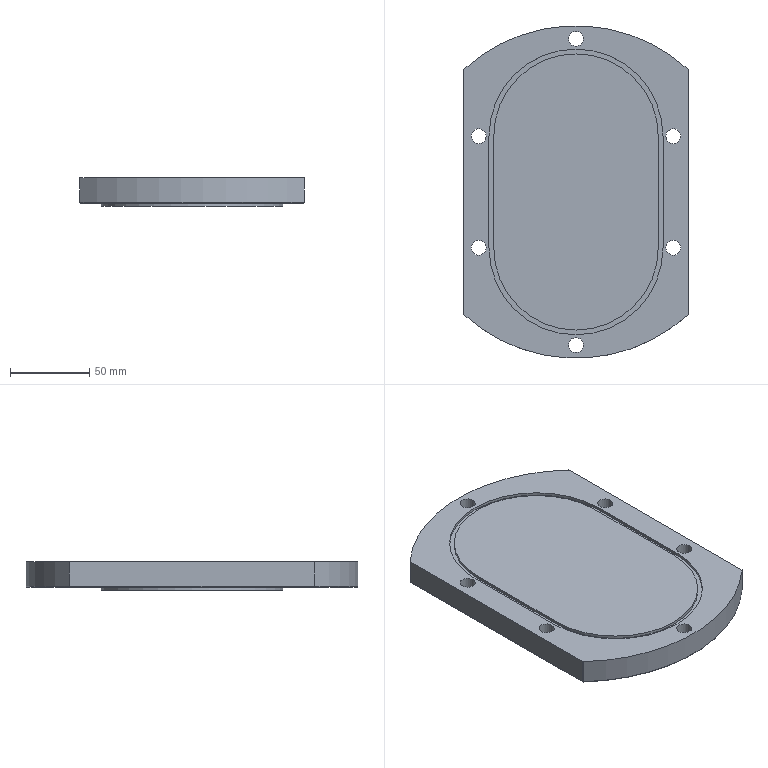Part | 1 solid | 52 faces | box 142 x 210 x 18 mm | volume 444849 mm3 | cylinder 24 | plane 17 | cone 6 | sphere 3 | torus 2 | commonest cylinder face diameters 9.5 x6 14 x6 1 x5 104 x2 110 x2 210 x2
STEP:
#1=CARTESIAN_POINT('',(71.,-77.356,0.));
#2=VERTEX_POINT('',#1);
#3=CARTESIAN_POINT('',(-70.837,-77.505,0.));
#4=VERTEX_POINT('',#3);
#5=CARTESIAN_POINT('',(0.,0.,0.));
#6=DIRECTION('',(0.,0.,-1.));
#7=DIRECTION('',(-1.,0.,0.));
#8=AXIS2_PLACEMENT_3D('',#5,#6,#7);
#9=CIRCLE('',#8,105.);
#10=EDGE_CURVE('',#2,#4,#9,.T.);
#11=ORIENTED_EDGE('',*,*,#10,.T.);
#12=CARTESIAN_POINT('',(-70.837,-77.505,-15.5));
#13=VERTEX_POINT('',#12);
#14=CARTESIAN_POINT('',(-70.837,-77.505,-16.));
#15=DIRECTION('',(0.,0.,1.));
#16=VECTOR('',#15,1000.);
#17=LINE('',#14,#16);
#18=EDGE_CURVE('',#4,#13,#17,.F.);
#19=ORIENTED_EDGE('',*,*,#18,.T.);
#20=CARTESIAN_POINT('',(71.,-77.356,-15.5));
#21=VERTEX_POINT('',#20);
#22=CARTESIAN_POINT('',(0.,0.,-15.5));
#23=DIRECTION('',(0.,0.,-1.));
#24=DIRECTION('',(-1.,0.,0.));
#25=AXIS2_PLACEMENT_3D('',#22,#23,#24);
#26=CIRCLE('',#25,105.);
#27=EDGE_CURVE('',#13,#21,#26,.F.);
#28=ORIENTED_EDGE('',*,*,#27,.T.);
#29=CARTESIAN_POINT('',(71.,-77.356,-16.));
#30=DIRECTION('',(0.,0.,1.));
#31=VECTOR('',#30,1000.);
#32=LINE('',#29,#31);
#33=EDGE_CURVE('',#21,#2,#32,.T.);
#34=ORIENTED_EDGE('',*,*,#33,.T.);
#35=EDGE_LOOP('',(#11,#19,#28,#34));
#36=FACE_BOUND('',#35,.T.);
#37=CARTESIAN_POINT('',(0.,0.,-16.));
#38=DIRECTION('',(0.,0.,1.));
#39=DIRECTION('',(1.,0.,0.));
#40=AXIS2_PLACEMENT_3D('',#37,#38,#39);
#41=CYLINDRICAL_SURFACE('',#40,105.);
#42=ADVANCED_FACE('',(#36),#41,.T.);
#43=CARTESIAN_POINT('',(-71.,-77.136,0.));
#44=VERTEX_POINT('',#43);
#45=CARTESIAN_POINT('',(-71.,77.136,0.));
#46=VERTEX_POINT('',#45);
#47=CARTESIAN_POINT('',(-71.,-77.356,0.));
#48=DIRECTION('',(0.,1.,0.));
#49=VECTOR('',#48,1000.);
#50=LINE('',#47,#49);
#51=EDGE_CURVE('',#44,#46,#50,.T.);
#52=ORIENTED_EDGE('',*,*,#51,.T.);
#53=CARTESIAN_POINT('',(-71.,77.136,-15.5));
#54=VERTEX_POINT('',#53);
#55=CARTESIAN_POINT('',(-71.,77.136,-16.));
#56=DIRECTION('',(0.,0.,1.));
#57=VECTOR('',#56,1000.);
#58=LINE('',#55,#57);
#59=EDGE_CURVE('',#46,#54,#58,.F.);
#60=ORIENTED_EDGE('',*,*,#59,.T.);
#61=CARTESIAN_POINT('',(-71.,-77.136,-15.5));
#62=VERTEX_POINT('',#61);
#63=CARTESIAN_POINT('',(-71.,-77.356,-15.5));
#64=DIRECTION('',(0.,1.,0.));
#65=VECTOR('',#64,1000.);
#66=LINE('',#63,#65);
#67=EDGE_CURVE('',#54,#62,#66,.F.);
#68=ORIENTED_EDGE('',*,*,#67,.T.);
#69=CARTESIAN_POINT('',(-71.,-77.136,-16.));
#70=DIRECTION('',(0.,0.,1.));
#71=VECTOR('',#70,1000.);
#72=LINE('',#69,#71);
#73=EDGE_CURVE('',#62,#44,#72,.T.);
#74=ORIENTED_EDGE('',*,*,#73,.T.);
#75=EDGE_LOOP('',(#52,#60,#68,#74));
#76=FACE_BOUND('',#75,.T.);
#77=CARTESIAN_POINT('',(-71.,-77.356,-16.));
#78=DIRECTION('',(1.,0.,0.));
#79=DIRECTION('',(0.,0.,-1.));
#80=AXIS2_PLACEMENT_3D('',#77,#78,#79);
#81=PLANE('',#80);
#82=ADVANCED_FACE('',(#76),#81,.F.);
#83=CARTESIAN_POINT('',(-70.837,77.505,0.));
#84=VERTEX_POINT('',#83);
#85=CARTESIAN_POINT('',(70.837,77.505,0.));
#86=VERTEX_POINT('',#85);
#87=CARTESIAN_POINT('',(0.,0.,0.));
#88=DIRECTION('',(0.,0.,-1.));
#89=DIRECTION('',(-1.,0.,0.));
#90=AXIS2_PLACEMENT_3D('',#87,#88,#89);
#91=CIRCLE('',#90,105.);
#92=EDGE_CURVE('',#84,#86,#91,.T.);
#93=ORIENTED_EDGE('',*,*,#92,.T.);
#94=CARTESIAN_POINT('',(70.837,77.505,-15.5));
#95=VERTEX_POINT('',#94);
#96=CARTESIAN_POINT('',(70.837,77.505,-16.));
#97=DIRECTION('',(0.,0.,1.));
#98=VECTOR('',#97,1000.);
#99=LINE('',#96,#98);
#100=EDGE_CURVE('',#86,#95,#99,.F.);
#101=ORIENTED_EDGE('',*,*,#100,.T.);
#102=CARTESIAN_POINT('',(-70.837,77.505,-15.5));
#103=VERTEX_POINT('',#102);
#104=CARTESIAN_POINT('',(0.,0.,-15.5));
#105=DIRECTION('',(0.,0.,-1.));
#106=DIRECTION('',(-1.,0.,0.));
#107=AXIS2_PLACEMENT_3D('',#104,#105,#106);
#108=CIRCLE('',#107,105.);
#109=EDGE_CURVE('',#95,#103,#108,.F.);
#110=ORIENTED_EDGE('',*,*,#109,.T.);
#111=CARTESIAN_POINT('',(-70.837,77.505,-16.));
#112=DIRECTION('',(0.,0.,1.));
#113=VECTOR('',#112,1000.);
#114=LINE('',#111,#113);
#115=EDGE_CURVE('',#103,#84,#114,.T.);
#116=ORIENTED_EDGE('',*,*,#115,.T.);
#117=EDGE_LOOP('',(#93,#101,#110,#116));
#118=FACE_BOUND('',#117,.T.);
#119=CARTESIAN_POINT('',(0.,0.,-16.));
#120=DIRECTION('',(0.,0.,1.));
#121=DIRECTION('',(1.,0.,0.));
#122=AXIS2_PLACEMENT_3D('',#119,#120,#121);
#123=CYLINDRICAL_SURFACE('',#122,105.);
#124=ADVANCED_FACE('',(#118),#123,.T.);
#125=CARTESIAN_POINT('',(71.,77.136,-15.5));
#126=VERTEX_POINT('',#125);
#127=CARTESIAN_POINT('',(71.,77.356,-15.5));
#128=DIRECTION('',(0.,-1.,0.));
#129=VECTOR('',#128,1000.);
#130=LINE('',#127,#129);
#131=EDGE_CURVE('',#21,#126,#130,.F.);
#132=ORIENTED_EDGE('',*,*,#131,.T.);
#133=CARTESIAN_POINT('',(71.,77.136,0.));
#134=VERTEX_POINT('',#133);
#135=CARTESIAN_POINT('',(71.,77.136,-16.));
#136=DIRECTION('',(0.,0.,1.));
#137=VECTOR('',#136,1000.);
#138=LINE('',#135,#137);
#139=EDGE_CURVE('',#126,#134,#138,.T.);
#140=ORIENTED_EDGE('',*,*,#139,.T.);
#141=CARTESIAN_POINT('',(71.,77.356,0.));
#142=DIRECTION('',(0.,-1.,0.));
#143=VECTOR('',#142,1000.);
#144=LINE('',#141,#143);
#145=EDGE_CURVE('',#134,#2,#144,.T.);
#146=ORIENTED_EDGE('',*,*,#145,.T.);
#147=ORIENTED_EDGE('',*,*,#33,.F.);
#148=EDGE_LOOP('',(#132,#140,#146,#147));
#149=FACE_BOUND('',#148,.T.);
#150=CARTESIAN_POINT('',(71.,77.356,-16.));
#151=DIRECTION('',(-1.,0.,0.));
#152=DIRECTION('',(0.,0.,1.));
#153=AXIS2_PLACEMENT_3D('',#150,#151,#152);
#154=PLANE('',#153);
#155=ADVANCED_FACE('',(#149),#154,.F.);
#156=CARTESIAN_POINT('',(-70.5,-77.136,-16.));
#157=VERTEX_POINT('',#156);
#158=CARTESIAN_POINT('',(-70.5,77.136,-16.));
#159=VERTEX_POINT('',#158);
#160=CARTESIAN_POINT('',(-70.5,77.356,-16.));
#161=DIRECTION('',(0.,1.,0.));
#162=VECTOR('',#161,1000.);
#163=LINE('',#160,#162);
#164=EDGE_CURVE('',#157,#159,#163,.T.);
#165=ORIENTED_EDGE('',*,*,#164,.T.);
#166=CARTESIAN_POINT('',(70.5,77.136,-16.));
#167=VERTEX_POINT('',#166);
#168=CARTESIAN_POINT('',(0.,0.,-16.));
#169=DIRECTION('',(0.,0.,-1.));
#170=DIRECTION('',(-1.,0.,0.));
#171=AXIS2_PLACEMENT_3D('',#168,#169,#170);
#172=CIRCLE('',#171,104.5);
#173=EDGE_CURVE('',#159,#167,#172,.T.);
#174=ORIENTED_EDGE('',*,*,#173,.T.);
#175=CARTESIAN_POINT('',(70.5,-77.136,-16.));
#176=VERTEX_POINT('',#175);
#177=CARTESIAN_POINT('',(70.5,-77.356,-16.));
#178=DIRECTION('',(0.,-1.,0.));
#179=VECTOR('',#178,1000.);
#180=LINE('',#177,#179);
#181=EDGE_CURVE('',#167,#176,#180,.T.);
#182=ORIENTED_EDGE('',*,*,#181,.T.);
#183=CARTESIAN_POINT('',(0.,0.,-16.));
#184=DIRECTION('',(0.,0.,-1.));
#185=DIRECTION('',(-1.,0.,0.));
#186=AXIS2_PLACEMENT_3D('',#183,#184,#185);
#187=CIRCLE('',#186,104.5);
#188=EDGE_CURVE('',#176,#157,#187,.T.);
#189=ORIENTED_EDGE('',*,*,#188,.T.);
#190=EDGE_LOOP('',(#165,#174,#182,#189));
#191=FACE_BOUND('',#190,.T.);
#192=CARTESIAN_POINT('',(-7.25,96.75,-16.));
#193=VERTEX_POINT('',#192);
#194=CARTESIAN_POINT('',(0.,96.75,-16.));
#195=DIRECTION('',(0.,0.,-1.));
#196=DIRECTION('',(-1.,0.,0.));
#197=AXIS2_PLACEMENT_3D('',#194,#195,#196);
#198=CIRCLE('',#197,7.25);
#199=EDGE_CURVE('',#193,#193,#198,.T.);
#200=ORIENTED_EDGE('',*,*,#199,.F.);
#201=EDGE_LOOP('',(#200));
#202=FACE_BOUND('',#201,.T.);
#203=CARTESIAN_POINT('',(54.25,35.25,-16.));
#204=VERTEX_POINT('',#203);
#205=CARTESIAN_POINT('',(61.5,35.25,-16.));
#206=DIRECTION('',(0.,0.,-1.));
#207=DIRECTION('',(-1.,0.,0.));
#208=AXIS2_PLACEMENT_3D('',#205,#206,#207);
#209=CIRCLE('',#208,7.25);
#210=EDGE_CURVE('',#204,#204,#209,.T.);
#211=ORIENTED_EDGE('',*,*,#210,.F.);
#212=EDGE_LOOP('',(#211));
#213=FACE_BOUND('',#212,.T.);
#214=CARTESIAN_POINT('',(-68.75,35.25,-16.));
#215=VERTEX_POINT('',#214);
#216=CARTESIAN_POINT('',(-61.5,35.25,-16.));
#217=DIRECTION('',(0.,0.,-1.));
#218=DIRECTION('',(-1.,0.,0.));
#219=AXIS2_PLACEMENT_3D('',#216,#217,#218);
#220=CIRCLE('',#219,7.25);
#221=EDGE_CURVE('',#215,#215,#220,.T.);
#222=ORIENTED_EDGE('',*,*,#221,.F.);
#223=EDGE_LOOP('',(#222));
#224=FACE_BOUND('',#223,.T.);
#225=CARTESIAN_POINT('',(-68.75,-35.25,-16.));
#226=VERTEX_POINT('',#225);
#227=CARTESIAN_POINT('',(-61.5,-35.25,-16.));
#228=DIRECTION('',(0.,0.,-1.));
#229=DIRECTION('',(-1.,0.,0.));
#230=AXIS2_PLACEMENT_3D('',#227,#228,#229);
#231=CIRCLE('',#230,7.25);
#232=EDGE_CURVE('',#226,#226,#231,.T.);
#233=ORIENTED_EDGE('',*,*,#232,.F.);
#234=EDGE_LOOP('',(#233));
#235=FACE_BOUND('',#234,.T.);
#236=CARTESIAN_POINT('',(54.25,-35.25,-16.));
#237=VERTEX_POINT('',#236);
#238=CARTESIAN_POINT('',(61.5,-35.25,-16.));
#239=DIRECTION('',(0.,0.,-1.));
#240=DIRECTION('',(-1.,0.,0.));
#241=AXIS2_PLACEMENT_3D('',#238,#239,#240);
#242=CIRCLE('',#241,7.25);
#243=EDGE_CURVE('',#237,#237,#242,.T.);
#244=ORIENTED_EDGE('',*,*,#243,.F.);
#245=EDGE_LOOP('',(#244));
#246=FACE_BOUND('',#245,.T.);
#247=CARTESIAN_POINT('',(-7.25,-96.75,-16.));
#248=VERTEX_POINT('',#247);
#249=CARTESIAN_POINT('',(0.,-96.75,-16.));
#250=DIRECTION('',(0.,0.,-1.));
#251=DIRECTION('',(-1.,0.,0.));
#252=AXIS2_PLACEMENT_3D('',#249,#250,#251);
#253=CIRCLE('',#252,7.25);
#254=EDGE_CURVE('',#248,#248,#253,.T.);
#255=ORIENTED_EDGE('',*,*,#254,.F.);
#256=EDGE_LOOP('',(#255));
#257=FACE_BOUND('',#256,.T.);
#258=CARTESIAN_POINT('',(-57.5,0.,-16.));
#259=VERTEX_POINT('',#258);
#260=CARTESIAN_POINT('',(0.,0.,-16.));
#261=DIRECTION('',(0.,0.,-1.));
#262=DIRECTION('',(-1.,0.,0.));
#263=AXIS2_PLACEMENT_3D('',#260,#261,#262);
#264=CIRCLE('',#263,57.5);
#265=EDGE_CURVE('',#259,#259,#264,.T.);
#266=ORIENTED_EDGE('',*,*,#265,.F.);
#267=EDGE_LOOP('',(#266));
#268=FACE_BOUND('',#267,.T.);
#269=CARTESIAN_POINT('',(0.,0.,-16.));
#270=DIRECTION('',(0.,0.,-1.));
#271=DIRECTION('',(-1.,0.,0.));
#272=AXIS2_PLACEMENT_3D('',#269,#270,#271);
#273=PLANE('',#272);
#274=ADVANCED_FACE('',(#191,#202,#213,#224,#235,#246,#257,#268),#273,.T.);
#275=CARTESIAN_POINT('',(-55.,35.25,0.));
#276=VERTEX_POINT('',#275);
#277=CARTESIAN_POINT('',(-55.,-35.25,0.));
#278=VERTEX_POINT('',#277);
#279=CARTESIAN_POINT('',(-55.,35.25,0.));
#280=DIRECTION('',(0.,-1.,0.));
#281=VECTOR('',#280,1000.);
#282=LINE('',#279,#281);
#283=EDGE_CURVE('',#276,#278,#282,.T.);
#284=ORIENTED_EDGE('',*,*,#283,.F.);
#285=CARTESIAN_POINT('',(55.,35.25,0.));
#286=VERTEX_POINT('',#285);
#287=CARTESIAN_POINT('',(0.,35.25,0.));
#288=DIRECTION('',(0.,0.,1.));
#289=DIRECTION('',(1.,0.,0.));
#290=AXIS2_PLACEMENT_3D('',#287,#288,#289);
#291=CIRCLE('',#290,55.);
#292=EDGE_CURVE('',#286,#276,#291,.T.);
#293=ORIENTED_EDGE('',*,*,#292,.F.);
#294=CARTESIAN_POINT('',(55.,-35.25,0.));
#295=VERTEX_POINT('',#294);
#296=CARTESIAN_POINT('',(55.,35.25,0.));
#297=DIRECTION('',(0.,1.,0.));
#298=VECTOR('',#297,1000.);
#299=LINE('',#296,#298);
#300=EDGE_CURVE('',#295,#286,#299,.T.);
#301=ORIENTED_EDGE('',*,*,#300,.F.);
#302=CARTESIAN_POINT('',(0.,-35.25,0.));
#303=DIRECTION('',(0.,0.,1.));
#304=DIRECTION('',(1.,0.,0.));
#305=AXIS2_PLACEMENT_3D('',#302,#303,#304);
#306=CIRCLE('',#305,55.);
#307=EDGE_CURVE('',#278,#295,#306,.T.);
#308=ORIENTED_EDGE('',*,*,#307,.F.);
#309=EDGE_LOOP('',(#284,#293,#301,#308));
#310=FACE_BOUND('',#309,.T.);
#311=CARTESIAN_POINT('',(-4.75,96.75,0.));
#312=VERTEX_POINT('',#311);
#313=CARTESIAN_POINT('',(0.,96.75,0.));
#314=DIRECTION('',(0.,0.,-1.));
#315=DIRECTION('',(-1.,0.,0.));
#316=AXIS2_PLACEMENT_3D('',#313,#314,#315);
#317=CIRCLE('',#316,4.75);
#318=EDGE_CURVE('',#312,#312,#317,.T.);
#319=ORIENTED_EDGE('',*,*,#318,.T.);
#320=EDGE_LOOP('',(#319));
#321=FACE_BOUND('',#320,.T.);
#322=CARTESIAN_POINT('',(56.75,35.25,0.));
#323=VERTEX_POINT('',#322);
#324=CARTESIAN_POINT('',(61.5,35.25,0.));
#325=DIRECTION('',(0.,0.,-1.));
#326=DIRECTION('',(-1.,0.,0.));
#327=AXIS2_PLACEMENT_3D('',#324,#325,#326);
#328=CIRCLE('',#327,4.75);
#329=EDGE_CURVE('',#323,#323,#328,.T.);
#330=ORIENTED_EDGE('',*,*,#329,.T.);
#331=EDGE_LOOP('',(#330));
#332=FACE_BOUND('',#331,.T.);
#333=CARTESIAN_POINT('',(-66.25,35.25,0.));
#334=VERTEX_POINT('',#333);
#335=CARTESIAN_POINT('',(-61.5,35.25,0.));
#336=DIRECTION('',(0.,0.,-1.));
#337=DIRECTION('',(-1.,0.,0.));
#338=AXIS2_PLACEMENT_3D('',#335,#336,#337);
#339=CIRCLE('',#338,4.75);
#340=EDGE_CURVE('',#334,#334,#339,.T.);
#341=ORIENTED_EDGE('',*,*,#340,.T.);
#342=EDGE_LOOP('',(#341));
#343=FACE_BOUND('',#342,.T.);
#344=CARTESIAN_POINT('',(-66.25,-35.25,0.));
#345=VERTEX_POINT('',#344);
#346=CARTESIAN_POINT('',(-61.5,-35.25,0.));
#347=DIRECTION('',(0.,0.,-1.));
#348=DIRECTION('',(-1.,0.,0.));
#349=AXIS2_PLACEMENT_3D('',#346,#347,#348);
#350=CIRCLE('',#349,4.75);
#351=EDGE_CURVE('',#345,#345,#350,.T.);
#352=ORIENTED_EDGE('',*,*,#351,.T.);
#353=EDGE_LOOP('',(#352));
#354=FACE_BOUND('',#353,.T.);
#355=CARTESIAN_POINT('',(56.75,-35.25,0.));
#356=VERTEX_POINT('',#355);
#357=CARTESIAN_POINT('',(61.5,-35.25,0.));
#358=DIRECTION('',(0.,0.,-1.));
#359=DIRECTION('',(-1.,0.,0.));
#360=AXIS2_PLACEMENT_3D('',#357,#358,#359);
#361=CIRCLE('',#360,4.75);
#362=EDGE_CURVE('',#356,#356,#361,.T.);
#363=ORIENTED_EDGE('',*,*,#362,.T.);
#364=EDGE_LOOP('',(#363));
#365=FACE_BOUND('',#364,.T.);
#366=CARTESIAN_POINT('',(-4.75,-96.75,0.));
#367=VERTEX_POINT('',#366);
#368=CARTESIAN_POINT('',(0.,-96.75,0.));
#369=DIRECTION('',(0.,0.,-1.));
#370=DIRECTION('',(-1.,0.,0.));
#371=AXIS2_PLACEMENT_3D('',#368,#369,#370);
#372=CIRCLE('',#371,4.75);
#373=EDGE_CURVE('',#367,#367,#372,.T.);
#374=ORIENTED_EDGE('',*,*,#373,.T.);
#375=EDGE_LOOP('',(#374));
#376=FACE_BOUND('',#375,.T.);
#377=ORIENTED_EDGE('',*,*,#145,.F.);
#378=CARTESIAN_POINT('',(70.5,77.136,0.));
#379=DIRECTION('',(0.,0.,-1.));
#380=DIRECTION('',(-1.,0.,0.));
#381=AXIS2_PLACEMENT_3D('',#378,#379,#380);
#382=CIRCLE('',#381,0.5);
#383=EDGE_CURVE('',#134,#86,#382,.F.);
#384=ORIENTED_EDGE('',*,*,#383,.T.);
#385=ORIENTED_EDGE('',*,*,#92,.F.);
#386=CARTESIAN_POINT('',(-70.5,77.136,0.));
#387=DIRECTION('',(0.,0.,-1.));
#388=DIRECTION('',(-1.,0.,0.));
#389=AXIS2_PLACEMENT_3D('',#386,#387,#388);
#390=CIRCLE('',#389,0.5);
#391=EDGE_CURVE('',#84,#46,#390,.F.);
#392=ORIENTED_EDGE('',*,*,#391,.T.);
#393=ORIENTED_EDGE('',*,*,#51,.F.);
#394=CARTESIAN_POINT('',(-70.5,-77.136,0.));
#395=DIRECTION('',(0.,0.,-1.));
#396=DIRECTION('',(-1.,0.,0.));
#397=AXIS2_PLACEMENT_3D('',#394,#395,#396);
#398=CIRCLE('',#397,0.5);
#399=EDGE_CURVE('',#44,#4,#398,.F.);
#400=ORIENTED_EDGE('',*,*,#399,.T.);
#401=ORIENTED_EDGE('',*,*,#10,.F.);
#402=EDGE_LOOP('',(#377,#384,#385,#392,#393,#400,#401));
#403=FACE_BOUND('',#402,.T.);
#404=CARTESIAN_POINT('',(0.,0.,0.));
#405=DIRECTION('',(0.,0.,-1.));
#406=DIRECTION('',(-1.,0.,0.));
#407=AXIS2_PLACEMENT_3D('',#404,#405,#406);
#408=PLANE('',#407);
#409=ADVANCED_FACE('',(#310,#321,#332,#343,#354,#365,#376,#403),#408,.F.);
#410=CARTESIAN_POINT('',(-57.5,0.,-18.));
#411=VERTEX_POINT('',#410);
#412=CARTESIAN_POINT('',(0.,0.,-18.));
#413=DIRECTION('',(0.,0.,-1.));
#414=DIRECTION('',(-1.,0.,0.));
#415=AXIS2_PLACEMENT_3D('',#412,#413,#414);
#416=CIRCLE('',#415,57.5);
#417=EDGE_CURVE('',#411,#411,#416,.T.);
#418=ORIENTED_EDGE('',*,*,#417,.F.);
#419=EDGE_LOOP('',(#418));
#420=FACE_BOUND('',#419,.T.);
#421=ORIENTED_EDGE('',*,*,#265,.T.);
#422=EDGE_LOOP('',(#421));
#423=FACE_BOUND('',#422,.T.);
#424=CARTESIAN_POINT('',(0.,0.,-18.));
#425=DIRECTION('',(0.,0.,1.));
#426=DIRECTION('',(1.,0.,0.));
#427=AXIS2_PLACEMENT_3D('',#424,#425,#426);
#428=CYLINDRICAL_SURFACE('',#427,57.5);
#429=ADVANCED_FACE('',(#420,#423),#428,.T.);
#430=ORIENTED_EDGE('',*,*,#417,.T.);
#431=EDGE_LOOP('',(#430));
#432=FACE_BOUND('',#431,.T.);
#433=CARTESIAN_POINT('',(0.,0.,-18.));
#434=DIRECTION('',(0.,0.,-1.));
#435=DIRECTION('',(-1.,0.,0.));
#436=AXIS2_PLACEMENT_3D('',#433,#434,#435);
#437=PLANE('',#436);
#438=ADVANCED_FACE('',(#432),#437,.T.);
#439=CARTESIAN_POINT('',(-4.75,-96.75,-7.5));
#440=VERTEX_POINT('',#439);
#441=CARTESIAN_POINT('',(0.,-96.75,-7.5));
#442=DIRECTION('',(0.,0.,-1.));
#443=DIRECTION('',(-1.,0.,0.));
#444=AXIS2_PLACEMENT_3D('',#441,#442,#443);
#445=CIRCLE('',#444,4.75);
#446=EDGE_CURVE('',#440,#440,#445,.T.);
#447=ORIENTED_EDGE('',*,*,#446,.T.);
#448=EDGE_LOOP('',(#447));
#449=FACE_BOUND('',#448,.T.);
#450=ORIENTED_EDGE('',*,*,#373,.F.);
#451=EDGE_LOOP('',(#450));
#452=FACE_BOUND('',#451,.T.);
#453=CARTESIAN_POINT('',(0.,-96.75,-16.));
#454=DIRECTION('',(0.,0.,-1.));
#455=DIRECTION('',(-1.,0.,0.));
#456=AXIS2_PLACEMENT_3D('',#453,#454,#455);
#457=CYLINDRICAL_SURFACE('',#456,4.75);
#458=ADVANCED_FACE('',(#449,#452),#457,.F.);
#459=ORIENTED_EDGE('',*,*,#446,.F.);
#460=EDGE_LOOP('',(#459));
#461=FACE_BOUND('',#460,.T.);
#462=CARTESIAN_POINT('',(-7.,-96.75,-7.5));
#463=VERTEX_POINT('',#462);
#464=CARTESIAN_POINT('',(0.,-96.75,-7.5));
#465=DIRECTION('',(0.,0.,-1.));
#466=DIRECTION('',(-1.,0.,0.));
#467=AXIS2_PLACEMENT_3D('',#464,#465,#466);
#468=CIRCLE('',#467,7.);
#469=EDGE_CURVE('',#463,#463,#468,.T.);
#470=ORIENTED_EDGE('',*,*,#469,.T.);
#471=EDGE_LOOP('',(#470));
#472=FACE_BOUND('',#471,.T.);
#473=CARTESIAN_POINT('',(-4.75,-96.75,-7.5));
#474=DIRECTION('',(0.,0.,1.));
#475=DIRECTION('',(1.,0.,0.));
#476=AXIS2_PLACEMENT_3D('',#473,#474,#475);
#477=PLANE('',#476);
#478=ADVANCED_FACE('',(#461,#472),#477,.F.);
#479=ORIENTED_EDGE('',*,*,#469,.F.);
#480=EDGE_LOOP('',(#479));
#481=FACE_BOUND('',#480,.T.);
#482=CARTESIAN_POINT('',(-7.,-96.75,-15.75));
#483=VERTEX_POINT('',#482);
#484=CARTESIAN_POINT('',(0.,-96.75,-15.75));
#485=DIRECTION('',(0.,0.,-1.));
#486=DIRECTION('',(-1.,0.,0.));
#487=AXIS2_PLACEMENT_3D('',#484,#485,#486);
#488=CIRCLE('',#487,7.);
#489=EDGE_CURVE('',#483,#483,#488,.T.);
#490=ORIENTED_EDGE('',*,*,#489,.T.);
#491=EDGE_LOOP('',(#490));
#492=FACE_BOUND('',#491,.T.);
#493=CARTESIAN_POINT('',(0.,-96.75,-16.));
#494=DIRECTION('',(0.,0.,-1.));
#495=DIRECTION('',(-1.,0.,0.));
#496=AXIS2_PLACEMENT_3D('',#493,#494,#495);
#497=CYLINDRICAL_SURFACE('',#496,7.);
#498=ADVANCED_FACE('',(#481,#492),#497,.F.);
#499=ORIENTED_EDGE('',*,*,#489,.F.);
#500=EDGE_LOOP('',(#499));
#501=FACE_BOUND('',#500,.T.);
#502=ORIENTED_EDGE('',*,*,#254,.T.);
#503=EDGE_LOOP('',(#502));
#504=FACE_BOUND('',#503,.T.);
#505=CARTESIAN_POINT('',(0.,-96.75,-16.));
#506=DIRECTION('',(0.,0.,-1.));
#507=DIRECTION('',(-1.,0.,0.));
#508=AXIS2_PLACEMENT_3D('',#505,#506,#507);
#509=CONICAL_SURFACE('',#508,7.25,0.7854);
#510=ADVANCED_FACE('',(#501,#504),#509,.F.);
#511=CARTESIAN_POINT('',(56.75,-35.25,-7.5));
#512=VERTEX_POINT('',#511);
#513=CARTESIAN_POINT('',(61.5,-35.25,-7.5));
#514=DIRECTION('',(0.,0.,-1.));
#515=DIRECTION('',(-1.,0.,0.));
#516=AXIS2_PLACEMENT_3D('',#513,#514,#515);
#517=CIRCLE('',#516,4.75);
#518=EDGE_CURVE('',#512,#512,#517,.T.);
#519=ORIENTED_EDGE('',*,*,#518,.T.);
#520=EDGE_LOOP('',(#519));
#521=FACE_BOUND('',#520,.T.);
#522=ORIENTED_EDGE('',*,*,#362,.F.);
#523=EDGE_LOOP('',(#522));
#524=FACE_BOUND('',#523,.T.);
#525=CARTESIAN_POINT('',(61.5,-35.25,-16.));
#526=DIRECTION('',(0.,0.,-1.));
#527=DIRECTION('',(-1.,0.,0.));
#528=AXIS2_PLACEMENT_3D('',#525,#526,#527);
#529=CYLINDRICAL_SURFACE('',#528,4.75);
#530=ADVANCED_FACE('',(#521,#524),#529,.F.);
#531=ORIENTED_EDGE('',*,*,#518,.F.);
#532=EDGE_LOOP('',(#531));
#533=FACE_BOUND('',#532,.T.);
#534=CARTESIAN_POINT('',(54.5,-35.25,-7.5));
#535=VERTEX_POINT('',#534);
#536=CARTESIAN_POINT('',(61.5,-35.25,-7.5));
#537=DIRECTION('',(0.,0.,-1.));
#538=DIRECTION('',(-1.,0.,0.));
#539=AXIS2_PLACEMENT_3D('',#536,#537,#538);
#540=CIRCLE('',#539,7.);
#541=EDGE_CURVE('',#535,#535,#540,.T.);
#542=ORIENTED_EDGE('',*,*,#541,.T.);
#543=EDGE_LOOP('',(#542));
#544=FACE_BOUND('',#543,.T.);
#545=CARTESIAN_POINT('',(56.75,-35.25,-7.5));
#546=DIRECTION('',(0.,0.,1.));
#547=DIRECTION('',(1.,0.,0.));
#548=AXIS2_PLACEMENT_3D('',#545,#546,#547);
#549=PLANE('',#548);
#550=ADVANCED_FACE('',(#533,#544),#549,.F.);
#551=ORIENTED_EDGE('',*,*,#541,.F.);
#552=EDGE_LOOP('',(#551));
#553=FACE_BOUND('',#552,.T.);
#554=CARTESIAN_POINT('',(54.5,-35.25,-15.75));
#555=VERTEX_POINT('',#554);
#556=CARTESIAN_POINT('',(61.5,-35.25,-15.75));
#557=DIRECTION('',(0.,0.,-1.));
#558=DIRECTION('',(-1.,0.,0.));
#559=AXIS2_PLACEMENT_3D('',#556,#557,#558);
#560=CIRCLE('',#559,7.);
#561=EDGE_CURVE('',#555,#555,#560,.T.);
#562=ORIENTED_EDGE('',*,*,#561,.T.);
#563=EDGE_LOOP('',(#562));
#564=FACE_BOUND('',#563,.T.);
#565=CARTESIAN_POINT('',(61.5,-35.25,-16.));
#566=DIRECTION('',(0.,0.,-1.));
#567=DIRECTION('',(-1.,0.,0.));
#568=AXIS2_PLACEMENT_3D('',#565,#566,#567);
#569=CYLINDRICAL_SURFACE('',#568,7.);
#570=ADVANCED_FACE('',(#553,#564),#569,.F.);
#571=ORIENTED_EDGE('',*,*,#561,.F.);
#572=EDGE_LOOP('',(#571));
#573=FACE_BOUND('',#572,.T.);
#574=ORIENTED_EDGE('',*,*,#243,.T.);
#575=EDGE_LOOP('',(#574));
#576=FACE_BOUND('',#575,.T.);
#577=CARTESIAN_POINT('',(61.5,-35.25,-16.));
#578=DIRECTION('',(0.,0.,-1.));
#579=DIRECTION('',(-1.,0.,0.));
#580=AXIS2_PLACEMENT_3D('',#577,#578,#579);
#581=CONICAL_SURFACE('',#580,7.25,0.7854);
#582=ADVANCED_FACE('',(#573,#576),#581,.F.);
#583=CARTESIAN_POINT('',(-66.25,-35.25,-7.5));
#584=VERTEX_POINT('',#583);
#585=CARTESIAN_POINT('',(-61.5,-35.25,-7.5));
#586=DIRECTION('',(0.,0.,-1.));
#587=DIRECTION('',(-1.,0.,0.));
#588=AXIS2_PLACEMENT_3D('',#585,#586,#587);
#589=CIRCLE('',#588,4.75);
#590=EDGE_CURVE('',#584,#584,#589,.T.);
#591=ORIENTED_EDGE('',*,*,#590,.T.);
#592=EDGE_LOOP('',(#591));
#593=FACE_BOUND('',#592,.T.);
#594=ORIENTED_EDGE('',*,*,#351,.F.);
#595=EDGE_LOOP('',(#594));
#596=FACE_BOUND('',#595,.T.);
#597=CARTESIAN_POINT('',(-61.5,-35.25,-16.));
#598=DIRECTION('',(0.,0.,-1.));
#599=DIRECTION('',(-1.,0.,0.));
#600=AXIS2_PLACEMENT_3D('',#597,#598,#599);
#601=CYLINDRICAL_SURFACE('',#600,4.75);
#602=ADVANCED_FACE('',(#593,#596),#601,.F.);
#603=ORIENTED_EDGE('',*,*,#590,.F.);
#604=EDGE_LOOP('',(#603));
#605=FACE_BOUND('',#604,.T.);
#606=CARTESIAN_POINT('',(-68.5,-35.25,-7.5));
#607=VERTEX_POINT('',#606);
#608=CARTESIAN_POINT('',(-61.5,-35.25,-7.5));
#609=DIRECTION('',(0.,0.,-1.));
#610=DIRECTION('',(-1.,0.,0.));
#611=AXIS2_PLACEMENT_3D('',#608,#609,#610);
#612=CIRCLE('',#611,7.);
#613=EDGE_CURVE('',#607,#607,#612,.T.);
#614=ORIENTED_EDGE('',*,*,#613,.T.);
#615=EDGE_LOOP('',(#614));
#616=FACE_BOUND('',#615,.T.);
#617=CARTESIAN_POINT('',(-66.25,-35.25,-7.5));
#618=DIRECTION('',(0.,0.,1.));
#619=DIRECTION('',(1.,0.,0.));
#620=AXIS2_PLACEMENT_3D('',#617,#618,#619);
#621=PLANE('',#620);
#622=ADVANCED_FACE('',(#605,#616),#621,.F.);
#623=ORIENTED_EDGE('',*,*,#613,.F.);
#624=EDGE_LOOP('',(#623));
#625=FACE_BOUND('',#624,.T.);
#626=CARTESIAN_POINT('',(-68.5,-35.25,-15.75));
#627=VERTEX_POINT('',#626);
#628=CARTESIAN_POINT('',(-61.5,-35.25,-15.75));
#629=DIRECTION('',(0.,0.,-1.));
#630=DIRECTION('',(-1.,0.,0.));
#631=AXIS2_PLACEMENT_3D('',#628,#629,#630);
#632=CIRCLE('',#631,7.);
#633=EDGE_CURVE('',#627,#627,#632,.T.);
#634=ORIENTED_EDGE('',*,*,#633,.T.);
#635=EDGE_LOOP('',(#634));
#636=FACE_BOUND('',#635,.T.);
#637=CARTESIAN_POINT('',(-61.5,-35.25,-16.));
#638=DIRECTION('',(0.,0.,-1.));
#639=DIRECTION('',(-1.,0.,0.));
#640=AXIS2_PLACEMENT_3D('',#637,#638,#639);
#641=CYLINDRICAL_SURFACE('',#640,7.);
#642=ADVANCED_FACE('',(#625,#636),#641,.F.);
#643=ORIENTED_EDGE('',*,*,#633,.F.);
#644=EDGE_LOOP('',(#643));
#645=FACE_BOUND('',#644,.T.);
#646=ORIENTED_EDGE('',*,*,#232,.T.);
#647=EDGE_LOOP('',(#646));
#648=FACE_BOUND('',#647,.T.);
#649=CARTESIAN_POINT('',(-61.5,-35.25,-16.));
#650=DIRECTION('',(0.,0.,-1.));
#651=DIRECTION('',(-1.,0.,0.));
#652=AXIS2_PLACEMENT_3D('',#649,#650,#651);
#653=CONICAL_SURFACE('',#652,7.25,0.7854);
#654=ADVANCED_FACE('',(#645,#648),#653,.F.);
#655=CARTESIAN_POINT('',(-66.25,35.25,-7.5));
#656=VERTEX_POINT('',#655);
#657=CARTESIAN_POINT('',(-61.5,35.25,-7.5));
#658=DIRECTION('',(0.,0.,-1.));
#659=DIRECTION('',(-1.,0.,0.));
#660=AXIS2_PLACEMENT_3D('',#657,#658,#659);
#661=CIRCLE('',#660,4.75);
#662=EDGE_CURVE('',#656,#656,#661,.T.);
#663=ORIENTED_EDGE('',*,*,#662,.T.);
#664=EDGE_LOOP('',(#663));
#665=FACE_BOUND('',#664,.T.);
#666=ORIENTED_EDGE('',*,*,#340,.F.);
#667=EDGE_LOOP('',(#666));
#668=FACE_BOUND('',#667,.T.);
#669=CARTESIAN_POINT('',(-61.5,35.25,-16.));
#670=DIRECTION('',(0.,0.,-1.));
#671=DIRECTION('',(-1.,0.,0.));
#672=AXIS2_PLACEMENT_3D('',#669,#670,#671);
#673=CYLINDRICAL_SURFACE('',#672,4.75);
#674=ADVANCED_FACE('',(#665,#668),#673,.F.);
#675=ORIENTED_EDGE('',*,*,#662,.F.);
#676=EDGE_LOOP('',(#675));
#677=FACE_BOUND('',#676,.T.);
#678=CARTESIAN_POINT('',(-68.5,35.25,-7.5));
#679=VERTEX_POINT('',#678);
#680=CARTESIAN_POINT('',(-61.5,35.25,-7.5));
#681=DIRECTION('',(0.,0.,-1.));
#682=DIRECTION('',(-1.,0.,0.));
#683=AXIS2_PLACEMENT_3D('',#680,#681,#682);
#684=CIRCLE('',#683,7.);
#685=EDGE_CURVE('',#679,#679,#684,.T.);
#686=ORIENTED_EDGE('',*,*,#685,.T.);
#687=EDGE_LOOP('',(#686));
#688=FACE_BOUND('',#687,.T.);
#689=CARTESIAN_POINT('',(-66.25,35.25,-7.5));
#690=DIRECTION('',(0.,0.,1.));
#691=DIRECTION('',(1.,0.,0.));
#692=AXIS2_PLACEMENT_3D('',#689,#690,#691);
#693=PLANE('',#692);
#694=ADVANCED_FACE('',(#677,#688),#693,.F.);
#695=ORIENTED_EDGE('',*,*,#685,.F.);
#696=EDGE_LOOP('',(#695));
#697=FACE_BOUND('',#696,.T.);
#698=CARTESIAN_POINT('',(-68.5,35.25,-15.75));
#699=VERTEX_POINT('',#698);
#700=CARTESIAN_POINT('',(-61.5,35.25,-15.75));
#701=DIRECTION('',(0.,0.,-1.));
#702=DIRECTION('',(-1.,0.,0.));
#703=AXIS2_PLACEMENT_3D('',#700,#701,#702);
#704=CIRCLE('',#703,7.);
#705=EDGE_CURVE('',#699,#699,#704,.T.);
#706=ORIENTED_EDGE('',*,*,#705,.T.);
#707=EDGE_LOOP('',(#706));
#708=FACE_BOUND('',#707,.T.);
#709=CARTESIAN_POINT('',(-61.5,35.25,-16.));
#710=DIRECTION('',(0.,0.,-1.));
#711=DIRECTION('',(-1.,0.,0.));
#712=AXIS2_PLACEMENT_3D('',#709,#710,#711);
#713=CYLINDRICAL_SURFACE('',#712,7.);
#714=ADVANCED_FACE('',(#697,#708),#713,.F.);
#715=ORIENTED_EDGE('',*,*,#705,.F.);
#716=EDGE_LOOP('',(#715));
#717=FACE_BOUND('',#716,.T.);
#718=ORIENTED_EDGE('',*,*,#221,.T.);
#719=EDGE_LOOP('',(#718));
#720=FACE_BOUND('',#719,.T.);
#721=CARTESIAN_POINT('',(-61.5,35.25,-16.));
#722=DIRECTION('',(0.,0.,-1.));
#723=DIRECTION('',(-1.,0.,0.));
#724=AXIS2_PLACEMENT_3D('',#721,#722,#723);
#725=CONICAL_SURFACE('',#724,7.25,0.7854);
#726=ADVANCED_FACE('',(#717,#720),#725,.F.);
#727=CARTESIAN_POINT('',(56.75,35.25,-7.5));
#728=VERTEX_POINT('',#727);
#729=CARTESIAN_POINT('',(61.5,35.25,-7.5));
#730=DIRECTION('',(0.,0.,-1.));
#731=DIRECTION('',(-1.,0.,0.));
#732=AXIS2_PLACEMENT_3D('',#729,#730,#731);
#733=CIRCLE('',#732,4.75);
#734=EDGE_CURVE('',#728,#728,#733,.T.);
#735=ORIENTED_EDGE('',*,*,#734,.T.);
#736=EDGE_LOOP('',(#735));
#737=FACE_BOUND('',#736,.T.);
#738=ORIENTED_EDGE('',*,*,#329,.F.);
#739=EDGE_LOOP('',(#738));
#740=FACE_BOUND('',#739,.T.);
#741=CARTESIAN_POINT('',(61.5,35.25,-16.));
#742=DIRECTION('',(0.,0.,-1.));
#743=DIRECTION('',(-1.,0.,0.));
#744=AXIS2_PLACEMENT_3D('',#741,#742,#743);
#745=CYLINDRICAL_SURFACE('',#744,4.75);
#746=ADVANCED_FACE('',(#737,#740),#745,.F.);
#747=ORIENTED_EDGE('',*,*,#734,.F.);
#748=EDGE_LOOP('',(#747));
#749=FACE_BOUND('',#748,.T.);
#750=CARTESIAN_POINT('',(54.5,35.25,-7.5));
#751=VERTEX_POINT('',#750);
#752=CARTESIAN_POINT('',(61.5,35.25,-7.5));
#753=DIRECTION('',(0.,0.,-1.));
#754=DIRECTION('',(-1.,0.,0.));
#755=AXIS2_PLACEMENT_3D('',#752,#753,#754);
#756=CIRCLE('',#755,7.);
#757=EDGE_CURVE('',#751,#751,#756,.T.);
#758=ORIENTED_EDGE('',*,*,#757,.T.);
#759=EDGE_LOOP('',(#758));
#760=FACE_BOUND('',#759,.T.);
#761=CARTESIAN_POINT('',(56.75,35.25,-7.5));
#762=DIRECTION('',(0.,0.,1.));
#763=DIRECTION('',(1.,0.,0.));
#764=AXIS2_PLACEMENT_3D('',#761,#762,#763);
#765=PLANE('',#764);
#766=ADVANCED_FACE('',(#749,#760),#765,.F.);
#767=ORIENTED_EDGE('',*,*,#757,.F.);
#768=EDGE_LOOP('',(#767));
#769=FACE_BOUND('',#768,.T.);
#770=CARTESIAN_POINT('',(54.5,35.25,-15.75));
#771=VERTEX_POINT('',#770);
#772=CARTESIAN_POINT('',(61.5,35.25,-15.75));
#773=DIRECTION('',(0.,0.,-1.));
#774=DIRECTION('',(-1.,0.,0.));
#775=AXIS2_PLACEMENT_3D('',#772,#773,#774);
#776=CIRCLE('',#775,7.);
#777=EDGE_CURVE('',#771,#771,#776,.T.);
#778=ORIENTED_EDGE('',*,*,#777,.T.);
#779=EDGE_LOOP('',(#778));
#780=FACE_BOUND('',#779,.T.);
#781=CARTESIAN_POINT('',(61.5,35.25,-16.));
#782=DIRECTION('',(0.,0.,-1.));
#783=DIRECTION('',(-1.,0.,0.));
#784=AXIS2_PLACEMENT_3D('',#781,#782,#783);
#785=CYLINDRICAL_SURFACE('',#784,7.);
#786=ADVANCED_FACE('',(#769,#780),#785,.F.);
#787=ORIENTED_EDGE('',*,*,#777,.F.);
#788=EDGE_LOOP('',(#787));
#789=FACE_BOUND('',#788,.T.);
#790=ORIENTED_EDGE('',*,*,#210,.T.);
#791=EDGE_LOOP('',(#790));
#792=FACE_BOUND('',#791,.T.);
#793=CARTESIAN_POINT('',(61.5,35.25,-16.));
#794=DIRECTION('',(0.,0.,-1.));
#795=DIRECTION('',(-1.,0.,0.));
#796=AXIS2_PLACEMENT_3D('',#793,#794,#795);
#797=CONICAL_SURFACE('',#796,7.25,0.7854);
#798=ADVANCED_FACE('',(#789,#792),#797,.F.);
#799=CARTESIAN_POINT('',(-4.75,96.75,-7.5));
#800=VERTEX_POINT('',#799);
#801=CARTESIAN_POINT('',(0.,96.75,-7.5));
#802=DIRECTION('',(0.,0.,-1.));
#803=DIRECTION('',(-1.,0.,0.));
#804=AXIS2_PLACEMENT_3D('',#801,#802,#803);
#805=CIRCLE('',#804,4.75);
#806=EDGE_CURVE('',#800,#800,#805,.T.);
#807=ORIENTED_EDGE('',*,*,#806,.T.);
#808=EDGE_LOOP('',(#807));
#809=FACE_BOUND('',#808,.T.);
#810=ORIENTED_EDGE('',*,*,#318,.F.);
#811=EDGE_LOOP('',(#810));
#812=FACE_BOUND('',#811,.T.);
#813=CARTESIAN_POINT('',(0.,96.75,-16.));
#814=DIRECTION('',(0.,0.,-1.));
#815=DIRECTION('',(-1.,0.,0.));
#816=AXIS2_PLACEMENT_3D('',#813,#814,#815);
#817=CYLINDRICAL_SURFACE('',#816,4.75);
#818=ADVANCED_FACE('',(#809,#812),#817,.F.);
#819=ORIENTED_EDGE('',*,*,#806,.F.);
#820=EDGE_LOOP('',(#819));
#821=FACE_BOUND('',#820,.T.);
#822=CARTESIAN_POINT('',(-7.,96.75,-7.5));
#823=VERTEX_POINT('',#822);
#824=CARTESIAN_POINT('',(0.,96.75,-7.5));
#825=DIRECTION('',(0.,0.,-1.));
#826=DIRECTION('',(-1.,0.,0.));
#827=AXIS2_PLACEMENT_3D('',#824,#825,#826);
#828=CIRCLE('',#827,7.);
#829=EDGE_CURVE('',#823,#823,#828,.T.);
#830=ORIENTED_EDGE('',*,*,#829,.T.);
#831=EDGE_LOOP('',(#830));
#832=FACE_BOUND('',#831,.T.);
#833=CARTESIAN_POINT('',(-4.75,96.75,-7.5));
#834=DIRECTION('',(0.,0.,1.));
#835=DIRECTION('',(1.,0.,0.));
#836=AXIS2_PLACEMENT_3D('',#833,#834,#835);
#837=PLANE('',#836);
#838=ADVANCED_FACE('',(#821,#832),#837,.F.);
#839=ORIENTED_EDGE('',*,*,#829,.F.);
#840=EDGE_LOOP('',(#839));
#841=FACE_BOUND('',#840,.T.);
#842=CARTESIAN_POINT('',(-7.,96.75,-15.75));
#843=VERTEX_POINT('',#842);
#844=CARTESIAN_POINT('',(0.,96.75,-15.75));
#845=DIRECTION('',(0.,0.,-1.));
#846=DIRECTION('',(-1.,0.,0.));
#847=AXIS2_PLACEMENT_3D('',#844,#845,#846);
#848=CIRCLE('',#847,7.);
#849=EDGE_CURVE('',#843,#843,#848,.T.);
#850=ORIENTED_EDGE('',*,*,#849,.T.);
#851=EDGE_LOOP('',(#850));
#852=FACE_BOUND('',#851,.T.);
#853=CARTESIAN_POINT('',(0.,96.75,-16.));
#854=DIRECTION('',(0.,0.,-1.));
#855=DIRECTION('',(-1.,0.,0.));
#856=AXIS2_PLACEMENT_3D('',#853,#854,#855);
#857=CYLINDRICAL_SURFACE('',#856,7.);
#858=ADVANCED_FACE('',(#841,#852),#857,.F.);
#859=ORIENTED_EDGE('',*,*,#849,.F.);
#860=EDGE_LOOP('',(#859));
#861=FACE_BOUND('',#860,.T.);
#862=ORIENTED_EDGE('',*,*,#199,.T.);
#863=EDGE_LOOP('',(#862));
#864=FACE_BOUND('',#863,.T.);
#865=CARTESIAN_POINT('',(0.,96.75,-16.));
#866=DIRECTION('',(0.,0.,-1.));
#867=DIRECTION('',(-1.,0.,0.));
#868=AXIS2_PLACEMENT_3D('',#865,#866,#867);
#869=CONICAL_SURFACE('',#868,7.25,0.7854);
#870=ADVANCED_FACE('',(#861,#864),#869,.F.);
#871=ORIENTED_EDGE('',*,*,#399,.F.);
#872=ORIENTED_EDGE('',*,*,#73,.F.);
#873=CARTESIAN_POINT('',(-70.5,-77.136,-15.5));
#874=DIRECTION('',(0.,0.,-1.));
#875=DIRECTION('',(-1.,0.,0.));
#876=AXIS2_PLACEMENT_3D('',#873,#874,#875);
#877=CIRCLE('',#876,0.5);
#878=EDGE_CURVE('',#13,#62,#877,.T.);
#879=ORIENTED_EDGE('',*,*,#878,.F.);
#880=ORIENTED_EDGE('',*,*,#18,.F.);
#881=EDGE_LOOP('',(#871,#872,#879,#880));
#882=FACE_BOUND('',#881,.T.);
#883=CARTESIAN_POINT('',(-70.5,-77.136,-16.));
#884=DIRECTION('',(0.,0.,1.));
#885=DIRECTION('',(1.,0.,0.));
#886=AXIS2_PLACEMENT_3D('',#883,#884,#885);
#887=CYLINDRICAL_SURFACE('',#886,0.5);
#888=ADVANCED_FACE('',(#882),#887,.T.);
#889=ORIENTED_EDGE('',*,*,#391,.F.);
#890=ORIENTED_EDGE('',*,*,#115,.F.);
#891=CARTESIAN_POINT('',(-70.5,77.136,-15.5));
#892=DIRECTION('',(0.,0.,-1.));
#893=DIRECTION('',(-1.,0.,0.));
#894=AXIS2_PLACEMENT_3D('',#891,#892,#893);
#895=CIRCLE('',#894,0.5);
#896=EDGE_CURVE('',#54,#103,#895,.T.);
#897=ORIENTED_EDGE('',*,*,#896,.F.);
#898=ORIENTED_EDGE('',*,*,#59,.F.);
#899=EDGE_LOOP('',(#889,#890,#897,#898));
#900=FACE_BOUND('',#899,.T.);
#901=CARTESIAN_POINT('',(-70.5,77.136,-16.));
#902=DIRECTION('',(0.,0.,1.));
#903=DIRECTION('',(1.,0.,0.));
#904=AXIS2_PLACEMENT_3D('',#901,#902,#903);
#905=CYLINDRICAL_SURFACE('',#904,0.5);
#906=ADVANCED_FACE('',(#900),#905,.T.);
#907=CARTESIAN_POINT('',(-70.5,-77.136,-15.5));
#908=DIRECTION('',(0.,-1.,0.));
#909=DIRECTION('',(0.,0.,1.));
#910=AXIS2_PLACEMENT_3D('',#907,#908,#909);
#911=CIRCLE('',#910,0.5);
#912=EDGE_CURVE('',#62,#157,#911,.T.);
#913=ORIENTED_EDGE('',*,*,#912,.F.);
#914=ORIENTED_EDGE('',*,*,#67,.F.);
#915=CARTESIAN_POINT('',(-70.5,77.136,-15.5));
#916=DIRECTION('',(0.,1.,0.));
#917=DIRECTION('',(0.,0.,-1.));
#918=AXIS2_PLACEMENT_3D('',#915,#916,#917);
#919=CIRCLE('',#918,0.5);
#920=EDGE_CURVE('',#159,#54,#919,.T.);
#921=ORIENTED_EDGE('',*,*,#920,.F.);
#922=ORIENTED_EDGE('',*,*,#164,.F.);
#923=EDGE_LOOP('',(#913,#914,#921,#922));
#924=FACE_BOUND('',#923,.T.);
#925=CARTESIAN_POINT('',(-70.5,0.,-15.5));
#926=DIRECTION('',(0.,-1.,0.));
#927=DIRECTION('',(0.,0.,1.));
#928=AXIS2_PLACEMENT_3D('',#925,#926,#927);
#929=CYLINDRICAL_SURFACE('',#928,0.5);
#930=ADVANCED_FACE('',(#924),#929,.T.);
#931=ORIENTED_EDGE('',*,*,#878,.T.);
#932=ORIENTED_EDGE('',*,*,#912,.T.);
#933=CARTESIAN_POINT('',(-70.5,-77.136,-15.5));
#934=DIRECTION('',(-0.7381,0.6746,0.));
#935=DIRECTION('',(0.6746,0.7381,0.));
#936=AXIS2_PLACEMENT_3D('',#933,#934,#935);
#937=CIRCLE('',#936,0.5);
#938=EDGE_CURVE('',#13,#157,#937,.F.);
#939=ORIENTED_EDGE('',*,*,#938,.F.);
#940=EDGE_LOOP('',(#931,#932,#939));
#941=FACE_BOUND('',#940,.T.);
#942=CARTESIAN_POINT('',(-70.5,-77.136,-15.5));
#943=DIRECTION('',(0.,0.,-1.));
#944=DIRECTION('',(-1.,0.,0.));
#945=AXIS2_PLACEMENT_3D('',#942,#943,#944);
#946=SPHERICAL_SURFACE('',#945,0.5);
#947=ADVANCED_FACE('',(#941),#946,.T.);
#948=ORIENTED_EDGE('',*,*,#920,.T.);
#949=ORIENTED_EDGE('',*,*,#896,.T.);
#950=CARTESIAN_POINT('',(-70.5,77.136,-15.5));
#951=DIRECTION('',(-0.7381,-0.6746,0.));
#952=DIRECTION('',(-0.6746,0.7381,0.));
#953=AXIS2_PLACEMENT_3D('',#950,#951,#952);
#954=CIRCLE('',#953,0.5);
#955=EDGE_CURVE('',#159,#103,#954,.F.);
#956=ORIENTED_EDGE('',*,*,#955,.F.);
#957=EDGE_LOOP('',(#948,#949,#956));
#958=FACE_BOUND('',#957,.T.);
#959=CARTESIAN_POINT('',(-70.5,77.136,-15.5));
#960=DIRECTION('',(0.,0.,-1.));
#961=DIRECTION('',(-1.,0.,0.));
#962=AXIS2_PLACEMENT_3D('',#959,#960,#961);
#963=SPHERICAL_SURFACE('',#962,0.5);
#964=ADVANCED_FACE('',(#958),#963,.T.);
#965=ORIENTED_EDGE('',*,*,#938,.T.);
#966=ORIENTED_EDGE('',*,*,#188,.F.);
#967=CARTESIAN_POINT('',(71.,-77.356,-15.5));
#968=CARTESIAN_POINT('',(71.,-77.356,-15.777));
#969=CARTESIAN_POINT('',(70.749,-77.246,-16.));
#970=CARTESIAN_POINT('',(70.5,-77.136,-16.));
#971=B_SPLINE_CURVE_WITH_KNOTS('',3,(#967,#968,#969,#970),.UNSPECIFIED.,.F.,.F.,(4,4),(0.,0.0008177),.UNSPECIFIED.);
#972=EDGE_CURVE('',#21,#176,#971,.T.);
#973=ORIENTED_EDGE('',*,*,#972,.F.);
#974=ORIENTED_EDGE('',*,*,#27,.F.);
#975=EDGE_LOOP('',(#965,#966,#973,#974));
#976=FACE_BOUND('',#975,.T.);
#977=CARTESIAN_POINT('',(0.,0.,-15.5));
#978=DIRECTION('',(0.,0.,-1.));
#979=DIRECTION('',(-1.,0.,0.));
#980=AXIS2_PLACEMENT_3D('',#977,#978,#979);
#981=TOROIDAL_SURFACE('',#980,104.5,0.5);
#982=ADVANCED_FACE('',(#976),#981,.T.);
#983=ORIENTED_EDGE('',*,*,#955,.T.);
#984=ORIENTED_EDGE('',*,*,#109,.F.);
#985=CARTESIAN_POINT('',(70.5,77.136,-15.5));
#986=DIRECTION('',(0.7381,-0.6746,0.));
#987=DIRECTION('',(-0.6746,-0.7381,0.));
#988=AXIS2_PLACEMENT_3D('',#985,#986,#987);
#989=CIRCLE('',#988,0.5);
#990=EDGE_CURVE('',#167,#95,#989,.T.);
#991=ORIENTED_EDGE('',*,*,#990,.F.);
#992=ORIENTED_EDGE('',*,*,#173,.F.);
#993=EDGE_LOOP('',(#983,#984,#991,#992));
#994=FACE_BOUND('',#993,.T.);
#995=CARTESIAN_POINT('',(0.,0.,-15.5));
#996=DIRECTION('',(0.,0.,-1.));
#997=DIRECTION('',(-1.,0.,0.));
#998=AXIS2_PLACEMENT_3D('',#995,#996,#997);
#999=TOROIDAL_SURFACE('',#998,104.5,0.5);
#1000=ADVANCED_FACE('',(#994),#999,.T.);
#1001=ORIENTED_EDGE('',*,*,#972,.T.);
#1002=ORIENTED_EDGE('',*,*,#181,.F.);
#1003=CARTESIAN_POINT('',(70.5,77.136,-15.5));
#1004=DIRECTION('',(0.,1.,0.));
#1005=DIRECTION('',(0.,0.,-1.));
#1006=AXIS2_PLACEMENT_3D('',#1003,#1004,#1005);
#1007=CIRCLE('',#1006,0.5);
#1008=EDGE_CURVE('',#126,#167,#1007,.T.);
#1009=ORIENTED_EDGE('',*,*,#1008,.F.);
#1010=ORIENTED_EDGE('',*,*,#131,.F.);
#1011=EDGE_LOOP('',(#1001,#1002,#1009,#1010));
#1012=FACE_BOUND('',#1011,.T.);
#1013=CARTESIAN_POINT('',(70.5,0.,-15.5));
#1014=DIRECTION('',(0.,1.,0.));
#1015=DIRECTION('',(0.,0.,-1.));
#1016=AXIS2_PLACEMENT_3D('',#1013,#1014,#1015);
#1017=CYLINDRICAL_SURFACE('',#1016,0.5);
#1018=ADVANCED_FACE('',(#1012),#1017,.T.);
#1019=ORIENTED_EDGE('',*,*,#1008,.T.);
#1020=ORIENTED_EDGE('',*,*,#990,.T.);
#1021=CARTESIAN_POINT('',(70.5,77.136,-15.5));
#1022=DIRECTION('',(0.,0.,-1.));
#1023=DIRECTION('',(-1.,0.,0.));
#1024=AXIS2_PLACEMENT_3D('',#1021,#1022,#1023);
#1025=CIRCLE('',#1024,0.5);
#1026=EDGE_CURVE('',#126,#95,#1025,.F.);
#1027=ORIENTED_EDGE('',*,*,#1026,.F.);
#1028=EDGE_LOOP('',(#1019,#1020,#1027));
#1029=FACE_BOUND('',#1028,.T.);
#1030=CARTESIAN_POINT('',(70.5,77.136,-15.5));
#1031=DIRECTION('',(0.,0.,-1.));
#1032=DIRECTION('',(-1.,0.,0.));
#1033=AXIS2_PLACEMENT_3D('',#1030,#1031,#1032);
#1034=SPHERICAL_SURFACE('',#1033,0.5);
#1035=ADVANCED_FACE('',(#1029),#1034,.T.);
#1036=ORIENTED_EDGE('',*,*,#1026,.T.);
#1037=ORIENTED_EDGE('',*,*,#100,.F.);
#1038=ORIENTED_EDGE('',*,*,#383,.F.);
#1039=ORIENTED_EDGE('',*,*,#139,.F.);
#1040=EDGE_LOOP('',(#1036,#1037,#1038,#1039));
#1041=FACE_BOUND('',#1040,.T.);
#1042=CARTESIAN_POINT('',(70.5,77.136,-16.));
#1043=DIRECTION('',(0.,0.,1.));
#1044=DIRECTION('',(1.,0.,0.));
#1045=AXIS2_PLACEMENT_3D('',#1042,#1043,#1044);
#1046=CYLINDRICAL_SURFACE('',#1045,0.5);
#1047=ADVANCED_FACE('',(#1041),#1046,.T.);
#1048=ORIENTED_EDGE('',*,*,#292,.T.);
#1049=CARTESIAN_POINT('',(-55.,35.25,-1.8));
#1050=VERTEX_POINT('',#1049);
#1051=CARTESIAN_POINT('',(-55.,35.25,-1.8));
#1052=DIRECTION('',(0.,0.,1.));
#1053=VECTOR('',#1052,1000.);
#1054=LINE('',#1051,#1053);
#1055=EDGE_CURVE('',#1050,#276,#1054,.T.);
#1056=ORIENTED_EDGE('',*,*,#1055,.F.);
#1057=CARTESIAN_POINT('',(55.,35.25,-1.8));
#1058=VERTEX_POINT('',#1057);
#1059=CARTESIAN_POINT('',(0.,35.25,-1.8));
#1060=DIRECTION('',(0.,0.,1.));
#1061=DIRECTION('',(1.,0.,0.));
#1062=AXIS2_PLACEMENT_3D('',#1059,#1060,#1061);
#1063=CIRCLE('',#1062,55.);
#1064=EDGE_CURVE('',#1058,#1050,#1063,.T.);
#1065=ORIENTED_EDGE('',*,*,#1064,.F.);
#1066=CARTESIAN_POINT('',(55.,35.25,-1.8));
#1067=DIRECTION('',(0.,0.,1.));
#1068=VECTOR('',#1067,1000.);
#1069=LINE('',#1066,#1068);
#1070=EDGE_CURVE('',#1058,#286,#1069,.T.);
#1071=ORIENTED_EDGE('',*,*,#1070,.T.);
#1072=EDGE_LOOP('',(#1048,#1056,#1065,#1071));
#1073=FACE_BOUND('',#1072,.T.);
#1074=CARTESIAN_POINT('',(0.,35.25,-1.8));
#1075=DIRECTION('',(0.,0.,1.));
#1076=DIRECTION('',(1.,0.,0.));
#1077=AXIS2_PLACEMENT_3D('',#1074,#1075,#1076);
#1078=CYLINDRICAL_SURFACE('',#1077,55.);
#1079=ADVANCED_FACE('',(#1073),#1078,.F.);
#1080=ORIENTED_EDGE('',*,*,#300,.T.);
#1081=ORIENTED_EDGE('',*,*,#1070,.F.);
#1082=CARTESIAN_POINT('',(55.,-35.25,-1.8));
#1083=VERTEX_POINT('',#1082);
#1084=CARTESIAN_POINT('',(55.,35.25,-1.8));
#1085=DIRECTION('',(0.,1.,0.));
#1086=VECTOR('',#1085,1000.);
#1087=LINE('',#1084,#1086);
#1088=EDGE_CURVE('',#1083,#1058,#1087,.T.);
#1089=ORIENTED_EDGE('',*,*,#1088,.F.);
#1090=CARTESIAN_POINT('',(55.,-35.25,-1.8));
#1091=DIRECTION('',(0.,0.,1.));
#1092=VECTOR('',#1091,1000.);
#1093=LINE('',#1090,#1092);
#1094=EDGE_CURVE('',#1083,#295,#1093,.T.);
#1095=ORIENTED_EDGE('',*,*,#1094,.T.);
#1096=EDGE_LOOP('',(#1080,#1081,#1089,#1095));
#1097=FACE_BOUND('',#1096,.T.);
#1098=CARTESIAN_POINT('',(55.,35.25,-1.8));
#1099=DIRECTION('',(1.,0.,0.));
#1100=DIRECTION('',(0.,0.,-1.));
#1101=AXIS2_PLACEMENT_3D('',#1098,#1099,#1100);
#1102=PLANE('',#1101);
#1103=ADVANCED_FACE('',(#1097),#1102,.F.);
#1104=ORIENTED_EDGE('',*,*,#307,.T.);
#1105=ORIENTED_EDGE('',*,*,#1094,.F.);
#1106=CARTESIAN_POINT('',(-55.,-35.25,-1.8));
#1107=VERTEX_POINT('',#1106);
#1108=CARTESIAN_POINT('',(0.,-35.25,-1.8));
#1109=DIRECTION('',(0.,0.,1.));
#1110=DIRECTION('',(1.,0.,0.));
#1111=AXIS2_PLACEMENT_3D('',#1108,#1109,#1110);
#1112=CIRCLE('',#1111,55.);
#1113=EDGE_CURVE('',#1107,#1083,#1112,.T.);
#1114=ORIENTED_EDGE('',*,*,#1113,.F.);
#1115=CARTESIAN_POINT('',(-55.,-35.25,-1.8));
#1116=DIRECTION('',(0.,0.,1.));
#1117=VECTOR('',#1116,1000.);
#1118=LINE('',#1115,#1117);
#1119=EDGE_CURVE('',#1107,#278,#1118,.T.);
#1120=ORIENTED_EDGE('',*,*,#1119,.T.);
#1121=EDGE_LOOP('',(#1104,#1105,#1114,#1120));
#1122=FACE_BOUND('',#1121,.T.);
#1123=CARTESIAN_POINT('',(0.,-35.25,-1.8));
#1124=DIRECTION('',(0.,0.,1.));
#1125=DIRECTION('',(1.,0.,0.));
#1126=AXIS2_PLACEMENT_3D('',#1123,#1124,#1125);
#1127=CYLINDRICAL_SURFACE('',#1126,55.);
#1128=ADVANCED_FACE('',(#1122),#1127,.F.);
#1129=ORIENTED_EDGE('',*,*,#283,.T.);
#1130=ORIENTED_EDGE('',*,*,#1119,.F.);
#1131=CARTESIAN_POINT('',(-55.,35.25,-1.8));
#1132=DIRECTION('',(0.,-1.,0.));
#1133=VECTOR('',#1132,1000.);
#1134=LINE('',#1131,#1133);
#1135=EDGE_CURVE('',#1050,#1107,#1134,.T.);
#1136=ORIENTED_EDGE('',*,*,#1135,.F.);
#1137=ORIENTED_EDGE('',*,*,#1055,.T.);
#1138=EDGE_LOOP('',(#1129,#1130,#1136,#1137));
#1139=FACE_BOUND('',#1138,.T.);
#1140=CARTESIAN_POINT('',(-55.,35.25,-1.8));
#1141=DIRECTION('',(-1.,0.,0.));
#1142=DIRECTION('',(0.,0.,1.));
#1143=AXIS2_PLACEMENT_3D('',#1140,#1141,#1142);
#1144=PLANE('',#1143);
#1145=ADVANCED_FACE('',(#1139),#1144,.F.);
#1146=CARTESIAN_POINT('',(52.,-35.25,-1.8));
#1147=VERTEX_POINT('',#1146);
#1148=CARTESIAN_POINT('',(52.,35.25,-1.8));
#1149=VERTEX_POINT('',#1148);
#1150=CARTESIAN_POINT('',(52.,35.25,-1.8));
#1151=DIRECTION('',(0.,1.,0.));
#1152=VECTOR('',#1151,1000.);
#1153=LINE('',#1150,#1152);
#1154=EDGE_CURVE('',#1147,#1149,#1153,.T.);
#1155=ORIENTED_EDGE('',*,*,#1154,.F.);
#1156=CARTESIAN_POINT('',(-52.,-35.25,-1.8));
#1157=VERTEX_POINT('',#1156);
#1158=CARTESIAN_POINT('',(0.,-35.25,-1.8));
#1159=DIRECTION('',(0.,0.,1.));
#1160=DIRECTION('',(1.,0.,0.));
#1161=AXIS2_PLACEMENT_3D('',#1158,#1159,#1160);
#1162=CIRCLE('',#1161,52.);
#1163=EDGE_CURVE('',#1157,#1147,#1162,.T.);
#1164=ORIENTED_EDGE('',*,*,#1163,.F.);
#1165=CARTESIAN_POINT('',(-52.,35.25,-1.8));
#1166=VERTEX_POINT('',#1165);
#1167=CARTESIAN_POINT('',(-52.,35.25,-1.8));
#1168=DIRECTION('',(0.,-1.,0.));
#1169=VECTOR('',#1168,1000.);
#1170=LINE('',#1167,#1169);
#1171=EDGE_CURVE('',#1166,#1157,#1170,.T.);
#1172=ORIENTED_EDGE('',*,*,#1171,.F.);
#1173=CARTESIAN_POINT('',(0.,35.25,-1.8));
#1174=DIRECTION('',(0.,0.,1.));
#1175=DIRECTION('',(1.,0.,0.));
#1176=AXIS2_PLACEMENT_3D('',#1173,#1174,#1175);
#1177=CIRCLE('',#1176,52.);
#1178=EDGE_CURVE('',#1149,#1166,#1177,.T.);
#1179=ORIENTED_EDGE('',*,*,#1178,.F.);
#1180=EDGE_LOOP('',(#1155,#1164,#1172,#1179));
#1181=FACE_BOUND('',#1180,.T.);
#1182=ORIENTED_EDGE('',*,*,#1064,.T.);
#1183=ORIENTED_EDGE('',*,*,#1135,.T.);
#1184=ORIENTED_EDGE('',*,*,#1113,.T.);
#1185=ORIENTED_EDGE('',*,*,#1088,.T.);
#1186=EDGE_LOOP('',(#1182,#1183,#1184,#1185));
#1187=FACE_BOUND('',#1186,.T.);
#1188=CARTESIAN_POINT('',(0.,35.25,-1.8));
#1189=DIRECTION('',(0.,0.,1.));
#1190=DIRECTION('',(1.,0.,0.));
#1191=AXIS2_PLACEMENT_3D('',#1188,#1189,#1190);
#1192=PLANE('',#1191);
#1193=ADVANCED_FACE('',(#1181,#1187),#1192,.T.);
#1194=CARTESIAN_POINT('',(52.,35.25,0.));
#1195=VERTEX_POINT('',#1194);
#1196=CARTESIAN_POINT('',(-52.,35.25,0.));
#1197=VERTEX_POINT('',#1196);
#1198=CARTESIAN_POINT('',(0.,35.25,0.));
#1199=DIRECTION('',(0.,0.,1.));
#1200=DIRECTION('',(1.,0.,0.));
#1201=AXIS2_PLACEMENT_3D('',#1198,#1199,#1200);
#1202=CIRCLE('',#1201,52.);
#1203=EDGE_CURVE('',#1195,#1197,#1202,.T.);
#1204=ORIENTED_EDGE('',*,*,#1203,.F.);
#1205=CARTESIAN_POINT('',(52.,35.25,-1.8));
#1206=DIRECTION('',(0.,0.,1.));
#1207=VECTOR('',#1206,1000.);
#1208=LINE('',#1205,#1207);
#1209=EDGE_CURVE('',#1149,#1195,#1208,.T.);
#1210=ORIENTED_EDGE('',*,*,#1209,.F.);
#1211=ORIENTED_EDGE('',*,*,#1178,.T.);
#1212=CARTESIAN_POINT('',(-52.,35.25,-1.8));
#1213=DIRECTION('',(0.,0.,1.));
#1214=VECTOR('',#1213,1000.);
#1215=LINE('',#1212,#1214);
#1216=EDGE_CURVE('',#1166,#1197,#1215,.T.);
#1217=ORIENTED_EDGE('',*,*,#1216,.T.);
#1218=EDGE_LOOP('',(#1204,#1210,#1211,#1217));
#1219=FACE_BOUND('',#1218,.T.);
#1220=CARTESIAN_POINT('',(0.,35.25,-1.8));
#1221=DIRECTION('',(0.,0.,1.));
#1222=DIRECTION('',(1.,0.,0.));
#1223=AXIS2_PLACEMENT_3D('',#1220,#1221,#1222);
#1224=CYLINDRICAL_SURFACE('',#1223,52.);
#1225=ADVANCED_FACE('',(#1219),#1224,.T.);
#1226=CARTESIAN_POINT('',(52.,-35.25,0.));
#1227=VERTEX_POINT('',#1226);
#1228=CARTESIAN_POINT('',(52.,35.25,0.));
#1229=DIRECTION('',(0.,1.,0.));
#1230=VECTOR('',#1229,1000.);
#1231=LINE('',#1228,#1230);
#1232=EDGE_CURVE('',#1227,#1195,#1231,.T.);
#1233=ORIENTED_EDGE('',*,*,#1232,.F.);
#1234=CARTESIAN_POINT('',(52.,-35.25,-1.8));
#1235=DIRECTION('',(0.,0.,1.));
#1236=VECTOR('',#1235,1000.);
#1237=LINE('',#1234,#1236);
#1238=EDGE_CURVE('',#1147,#1227,#1237,.T.);
#1239=ORIENTED_EDGE('',*,*,#1238,.F.);
#1240=ORIENTED_EDGE('',*,*,#1154,.T.);
#1241=ORIENTED_EDGE('',*,*,#1209,.T.);
#1242=EDGE_LOOP('',(#1233,#1239,#1240,#1241));
#1243=FACE_BOUND('',#1242,.T.);
#1244=CARTESIAN_POINT('',(52.,35.25,-1.8));
#1245=DIRECTION('',(1.,0.,0.));
#1246=DIRECTION('',(0.,0.,-1.));
#1247=AXIS2_PLACEMENT_3D('',#1244,#1245,#1246);
#1248=PLANE('',#1247);
#1249=ADVANCED_FACE('',(#1243),#1248,.T.);
#1250=CARTESIAN_POINT('',(-52.,-35.25,0.));
#1251=VERTEX_POINT('',#1250);
#1252=CARTESIAN_POINT('',(0.,-35.25,0.));
#1253=DIRECTION('',(0.,0.,1.));
#1254=DIRECTION('',(1.,0.,0.));
#1255=AXIS2_PLACEMENT_3D('',#1252,#1253,#1254);
#1256=CIRCLE('',#1255,52.);
#1257=EDGE_CURVE('',#1251,#1227,#1256,.T.);
#1258=ORIENTED_EDGE('',*,*,#1257,.F.);
#1259=CARTESIAN_POINT('',(-52.,-35.25,-1.8));
#1260=DIRECTION('',(0.,0.,1.));
#1261=VECTOR('',#1260,1000.);
#1262=LINE('',#1259,#1261);
#1263=EDGE_CURVE('',#1157,#1251,#1262,.T.);
#1264=ORIENTED_EDGE('',*,*,#1263,.F.);
#1265=ORIENTED_EDGE('',*,*,#1163,.T.);
#1266=ORIENTED_EDGE('',*,*,#1238,.T.);
#1267=EDGE_LOOP('',(#1258,#1264,#1265,#1266));
#1268=FACE_BOUND('',#1267,.T.);
#1269=CARTESIAN_POINT('',(0.,-35.25,-1.8));
#1270=DIRECTION('',(0.,0.,1.));
#1271=DIRECTION('',(1.,0.,0.));
#1272=AXIS2_PLACEMENT_3D('',#1269,#1270,#1271);
#1273=CYLINDRICAL_SURFACE('',#1272,52.);
#1274=ADVANCED_FACE('',(#1268),#1273,.T.);
#1275=CARTESIAN_POINT('',(-52.,35.25,0.));
#1276=DIRECTION('',(0.,-1.,0.));
#1277=VECTOR('',#1276,1000.);
#1278=LINE('',#1275,#1277);
#1279=EDGE_CURVE('',#1197,#1251,#1278,.T.);
#1280=ORIENTED_EDGE('',*,*,#1279,.F.);
#1281=ORIENTED_EDGE('',*,*,#1216,.F.);
#1282=ORIENTED_EDGE('',*,*,#1171,.T.);
#1283=ORIENTED_EDGE('',*,*,#1263,.T.);
#1284=EDGE_LOOP('',(#1280,#1281,#1282,#1283));
#1285=FACE_BOUND('',#1284,.T.);
#1286=CARTESIAN_POINT('',(-52.,35.25,-1.8));
#1287=DIRECTION('',(-1.,0.,0.));
#1288=DIRECTION('',(0.,0.,1.));
#1289=AXIS2_PLACEMENT_3D('',#1286,#1287,#1288);
#1290=PLANE('',#1289);
#1291=ADVANCED_FACE('',(#1285),#1290,.T.);
#1292=ORIENTED_EDGE('',*,*,#1203,.T.);
#1293=ORIENTED_EDGE('',*,*,#1279,.T.);
#1294=ORIENTED_EDGE('',*,*,#1257,.T.);
#1295=ORIENTED_EDGE('',*,*,#1232,.T.);
#1296=EDGE_LOOP('',(#1292,#1293,#1294,#1295));
#1297=FACE_BOUND('',#1296,.T.);
#1298=CARTESIAN_POINT('',(0.,0.,0.));
#1299=DIRECTION('',(0.,0.,-1.));
#1300=DIRECTION('',(-1.,0.,0.));
#1301=AXIS2_PLACEMENT_3D('',#1298,#1299,#1300);
#1302=PLANE('',#1301);
#1303=ADVANCED_FACE('',(#1297),#1302,.F.);
#1304=CLOSED_SHELL('',(#42,#82,#124,#155,#274,#409,#429,#438,#458,#478,#498,#510,#530,#550,#570,#582,#602,#622,#642,#654,#674,#694,#714,#726,#746,#766,#786,#798,#818,#838,#858,#870,#888,#906,#930,#947,#964,#982,#1000,#1018,#1035,#1047,#1079,#1103,#1128,#1145,#1193,#1225,#1249,#1274,#1291,#1303));
#1305=MANIFOLD_SOLID_BREP('',#1304);
#1306=(LENGTH_UNIT()NAMED_UNIT(*)SI_UNIT(.MILLI.,.METRE.));
#1307=UNCERTAINTY_MEASURE_WITH_UNIT(LENGTH_MEASURE(0.0508),#1306,'','');
#1308=(NAMED_UNIT(*)PLANE_ANGLE_UNIT()SI_UNIT($,.RADIAN.));
#1309=(NAMED_UNIT(*)SI_UNIT($,.STERADIAN.)SOLID_ANGLE_UNIT());
#1310=(GEOMETRIC_REPRESENTATION_CONTEXT(3)GLOBAL_UNCERTAINTY_ASSIGNED_CONTEXT((#1307))GLOBAL_UNIT_ASSIGNED_CONTEXT((#1306,#1308,#1309))REPRESENTATION_CONTEXT('',''));
#1311=ADVANCED_BREP_SHAPE_REPRESENTATION('',(#1305),#1310);